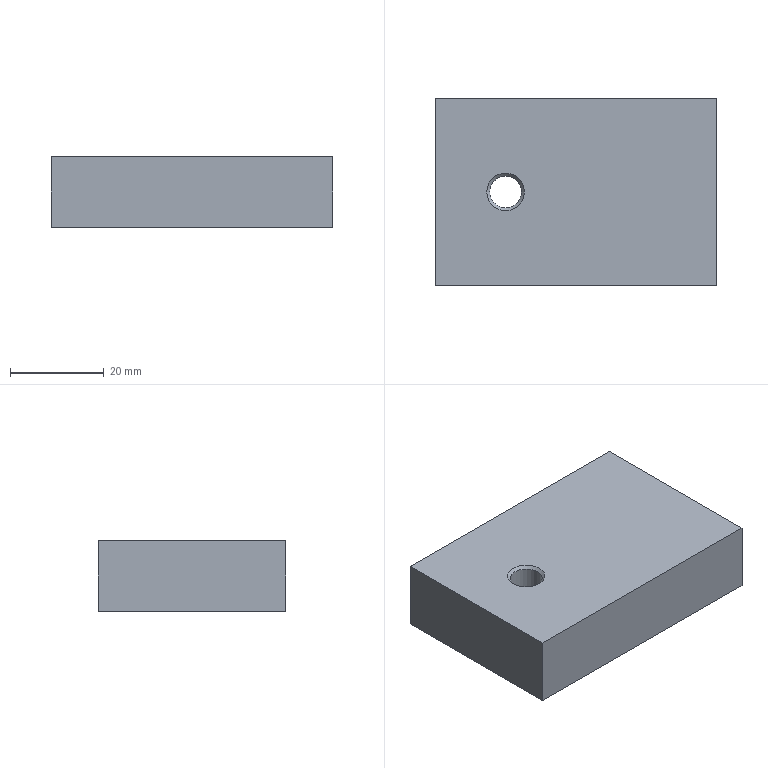Part | NX | features DATUM_CSYS 2, BLOCK 1, HOLE PACKAGE 1, SIMPLE HOLE 1, SKETCH 1, SYMBOLIC_THREAD 1 | 1 solid | 9 faces | box 60 x 40 x 15 mm | volume 35447 mm3 | plane 6 | cone 2 | cylinder 1 | commonest cylinder face diameters 6.8 x1
STEP:
#1=CARTESIAN_POINT('',(19.,20.,15.));
#2=VERTEX_POINT('',#1);
#3=CARTESIAN_POINT('',(15.,20.,15.));
#4=DIRECTION('',(0.,0.,1.));
#5=DIRECTION('',(1.,0.,0.));
#6=AXIS2_PLACEMENT_3D('',#3,#4,#5);
#7=CIRCLE('',#6,4.);
#8=EDGE_CURVE('',#2,#2,#7,.F.);
#9=ORIENTED_EDGE('',*,*,#8,.T.);
#10=EDGE_LOOP('',(#9));
#11=FACE_BOUND('',#10,.T.);
#12=CARTESIAN_POINT('',(60.,0.,15.));
#13=VERTEX_POINT('',#12);
#14=CARTESIAN_POINT('',(0.,0.,15.));
#15=VERTEX_POINT('',#14);
#16=CARTESIAN_POINT('',(30.,0.,15.));
#17=DIRECTION('',(-1.,0.,0.));
#18=VECTOR('',#17,1000.);
#19=LINE('',#16,#18);
#20=EDGE_CURVE('',#13,#15,#19,.T.);
#21=ORIENTED_EDGE('',*,*,#20,.F.);
#22=CARTESIAN_POINT('',(60.,40.,15.));
#23=VERTEX_POINT('',#22);
#24=CARTESIAN_POINT('',(60.,20.,15.));
#25=DIRECTION('',(0.,-1.,0.));
#26=VECTOR('',#25,1000.);
#27=LINE('',#24,#26);
#28=EDGE_CURVE('',#23,#13,#27,.T.);
#29=ORIENTED_EDGE('',*,*,#28,.F.);
#30=CARTESIAN_POINT('',(0.,40.,15.));
#31=VERTEX_POINT('',#30);
#32=CARTESIAN_POINT('',(30.,40.,15.));
#33=DIRECTION('',(1.,0.,0.));
#34=VECTOR('',#33,1000.);
#35=LINE('',#32,#34);
#36=EDGE_CURVE('',#31,#23,#35,.T.);
#37=ORIENTED_EDGE('',*,*,#36,.F.);
#38=CARTESIAN_POINT('',(0.,20.,15.));
#39=DIRECTION('',(0.,1.,0.));
#40=VECTOR('',#39,1000.);
#41=LINE('',#38,#40);
#42=EDGE_CURVE('',#15,#31,#41,.T.);
#43=ORIENTED_EDGE('',*,*,#42,.F.);
#44=EDGE_LOOP('',(#21,#29,#37,#43));
#45=FACE_BOUND('',#44,.T.);
#46=CARTESIAN_POINT('',(30.,20.,15.));
#47=DIRECTION('',(0.,0.,1.));
#48=DIRECTION('',(1.,0.,0.));
#49=AXIS2_PLACEMENT_3D('',#46,#47,#48);
#50=PLANE('',#49);
#51=ADVANCED_FACE('',(#11,#45),#50,.T.);
#52=CARTESIAN_POINT('',(60.,0.,0.));
#53=VERTEX_POINT('',#52);
#54=CARTESIAN_POINT('',(60.,0.,0.));
#55=DIRECTION('',(0.,0.,1.));
#56=VECTOR('',#55,1000.);
#57=LINE('',#54,#56);
#58=EDGE_CURVE('',#53,#13,#57,.T.);
#59=ORIENTED_EDGE('',*,*,#58,.T.);
#60=ORIENTED_EDGE('',*,*,#20,.T.);
#61=CARTESIAN_POINT('',(0.,0.,0.));
#62=VERTEX_POINT('',#61);
#63=CARTESIAN_POINT('',(0.,0.,0.));
#64=DIRECTION('',(0.,0.,1.));
#65=VECTOR('',#64,1000.);
#66=LINE('',#63,#65);
#67=EDGE_CURVE('',#62,#15,#66,.T.);
#68=ORIENTED_EDGE('',*,*,#67,.F.);
#69=CARTESIAN_POINT('',(30.,0.,0.));
#70=DIRECTION('',(1.,0.,0.));
#71=VECTOR('',#70,1000.);
#72=LINE('',#69,#71);
#73=EDGE_CURVE('',#62,#53,#72,.T.);
#74=ORIENTED_EDGE('',*,*,#73,.T.);
#75=EDGE_LOOP('',(#59,#60,#68,#74));
#76=FACE_BOUND('',#75,.T.);
#77=CARTESIAN_POINT('',(30.,0.,0.));
#78=DIRECTION('',(0.,-1.,0.));
#79=DIRECTION('',(0.,0.,-1.));
#80=AXIS2_PLACEMENT_3D('',#77,#78,#79);
#81=PLANE('',#80);
#82=ADVANCED_FACE('',(#76),#81,.T.);
#83=ORIENTED_EDGE('',*,*,#67,.T.);
#84=ORIENTED_EDGE('',*,*,#42,.T.);
#85=CARTESIAN_POINT('',(0.,40.,0.));
#86=VERTEX_POINT('',#85);
#87=CARTESIAN_POINT('',(0.,40.,0.));
#88=DIRECTION('',(0.,0.,1.));
#89=VECTOR('',#88,1000.);
#90=LINE('',#87,#89);
#91=EDGE_CURVE('',#86,#31,#90,.T.);
#92=ORIENTED_EDGE('',*,*,#91,.F.);
#93=CARTESIAN_POINT('',(0.,20.,0.));
#94=DIRECTION('',(0.,-1.,0.));
#95=VECTOR('',#94,1000.);
#96=LINE('',#93,#95);
#97=EDGE_CURVE('',#86,#62,#96,.T.);
#98=ORIENTED_EDGE('',*,*,#97,.T.);
#99=EDGE_LOOP('',(#83,#84,#92,#98));
#100=FACE_BOUND('',#99,.T.);
#101=CARTESIAN_POINT('',(0.,20.,0.));
#102=DIRECTION('',(-1.,0.,0.));
#103=DIRECTION('',(0.,0.,1.));
#104=AXIS2_PLACEMENT_3D('',#101,#102,#103);
#105=PLANE('',#104);
#106=ADVANCED_FACE('',(#100),#105,.T.);
#107=ORIENTED_EDGE('',*,*,#91,.T.);
#108=ORIENTED_EDGE('',*,*,#36,.T.);
#109=CARTESIAN_POINT('',(60.,40.,0.));
#110=VERTEX_POINT('',#109);
#111=CARTESIAN_POINT('',(60.,40.,0.));
#112=DIRECTION('',(0.,0.,1.));
#113=VECTOR('',#112,1000.);
#114=LINE('',#111,#113);
#115=EDGE_CURVE('',#110,#23,#114,.T.);
#116=ORIENTED_EDGE('',*,*,#115,.F.);
#117=CARTESIAN_POINT('',(30.,40.,0.));
#118=DIRECTION('',(-1.,0.,0.));
#119=VECTOR('',#118,1000.);
#120=LINE('',#117,#119);
#121=EDGE_CURVE('',#110,#86,#120,.T.);
#122=ORIENTED_EDGE('',*,*,#121,.T.);
#123=EDGE_LOOP('',(#107,#108,#116,#122));
#124=FACE_BOUND('',#123,.T.);
#125=CARTESIAN_POINT('',(30.,40.,0.));
#126=DIRECTION('',(0.,1.,0.));
#127=DIRECTION('',(0.,0.,1.));
#128=AXIS2_PLACEMENT_3D('',#125,#126,#127);
#129=PLANE('',#128);
#130=ADVANCED_FACE('',(#124),#129,.T.);
#131=CARTESIAN_POINT('',(11.,20.,0.));
#132=VERTEX_POINT('',#131);
#133=CARTESIAN_POINT('',(15.,20.,0.));
#134=DIRECTION('',(0.,0.,-1.));
#135=DIRECTION('',(-1.,0.,0.));
#136=AXIS2_PLACEMENT_3D('',#133,#134,#135);
#137=CIRCLE('',#136,4.);
#138=EDGE_CURVE('',#132,#132,#137,.F.);
#139=ORIENTED_EDGE('',*,*,#138,.T.);
#140=EDGE_LOOP('',(#139));
#141=FACE_BOUND('',#140,.T.);
#142=CARTESIAN_POINT('',(60.,20.,0.));
#143=DIRECTION('',(0.,1.,0.));
#144=VECTOR('',#143,1000.);
#145=LINE('',#142,#144);
#146=EDGE_CURVE('',#53,#110,#145,.T.);
#147=ORIENTED_EDGE('',*,*,#146,.F.);
#148=ORIENTED_EDGE('',*,*,#73,.F.);
#149=ORIENTED_EDGE('',*,*,#97,.F.);
#150=ORIENTED_EDGE('',*,*,#121,.F.);
#151=EDGE_LOOP('',(#147,#148,#149,#150));
#152=FACE_BOUND('',#151,.T.);
#153=CARTESIAN_POINT('',(30.,20.,0.));
#154=DIRECTION('',(0.,0.,-1.));
#155=DIRECTION('',(-1.,0.,0.));
#156=AXIS2_PLACEMENT_3D('',#153,#154,#155);
#157=PLANE('',#156);
#158=ADVANCED_FACE('',(#141,#152),#157,.T.);
#159=ORIENTED_EDGE('',*,*,#146,.T.);
#160=ORIENTED_EDGE('',*,*,#115,.T.);
#161=ORIENTED_EDGE('',*,*,#28,.T.);
#162=ORIENTED_EDGE('',*,*,#58,.F.);
#163=EDGE_LOOP('',(#159,#160,#161,#162));
#164=FACE_BOUND('',#163,.T.);
#165=CARTESIAN_POINT('',(60.,20.,0.));
#166=DIRECTION('',(1.,0.,0.));
#167=DIRECTION('',(0.,0.,-1.));
#168=AXIS2_PLACEMENT_3D('',#165,#166,#167);
#169=PLANE('',#168);
#170=ADVANCED_FACE('',(#164),#169,.T.);
#171=CARTESIAN_POINT('',(11.6,20.,0.6));
#172=VERTEX_POINT('',#171);
#173=CARTESIAN_POINT('',(15.,20.,0.6));
#174=DIRECTION('',(0.,0.,-1.));
#175=DIRECTION('',(-1.,0.,0.));
#176=AXIS2_PLACEMENT_3D('',#173,#174,#175);
#177=CIRCLE('',#176,3.4);
#178=EDGE_CURVE('',#172,#172,#177,.T.);
#179=ORIENTED_EDGE('',*,*,#178,.T.);
#180=EDGE_LOOP('',(#179));
#181=FACE_BOUND('',#180,.T.);
#182=CARTESIAN_POINT('',(18.4,20.,14.4));
#183=VERTEX_POINT('',#182);
#184=CARTESIAN_POINT('',(15.,20.,14.4));
#185=DIRECTION('',(0.,0.,1.));
#186=DIRECTION('',(1.,0.,0.));
#187=AXIS2_PLACEMENT_3D('',#184,#185,#186);
#188=CIRCLE('',#187,3.4);
#189=EDGE_CURVE('',#183,#183,#188,.T.);
#190=ORIENTED_EDGE('',*,*,#189,.T.);
#191=EDGE_LOOP('',(#190));
#192=FACE_BOUND('',#191,.T.);
#193=CARTESIAN_POINT('',(15.,20.,15.));
#194=DIRECTION('',(0.,0.,-1.));
#195=DIRECTION('',(-1.,0.,0.));
#196=AXIS2_PLACEMENT_3D('',#193,#194,#195);
#197=CYLINDRICAL_SURFACE('',#196,3.4);
#198=ADVANCED_FACE('',(#181,#192),#197,.F.);
#199=ORIENTED_EDGE('',*,*,#189,.F.);
#200=EDGE_LOOP('',(#199));
#201=FACE_BOUND('',#200,.T.);
#202=ORIENTED_EDGE('',*,*,#8,.F.);
#203=EDGE_LOOP('',(#202));
#204=FACE_BOUND('',#203,.T.);
#205=CARTESIAN_POINT('',(15.,20.,15.));
#206=DIRECTION('',(0.,0.,1.));
#207=DIRECTION('',(1.,0.,0.));
#208=AXIS2_PLACEMENT_3D('',#205,#206,#207);
#209=CONICAL_SURFACE('',#208,4.,0.7854);
#210=ADVANCED_FACE('',(#201,#204),#209,.F.);
#211=ORIENTED_EDGE('',*,*,#138,.F.);
#212=EDGE_LOOP('',(#211));
#213=FACE_BOUND('',#212,.T.);
#214=ORIENTED_EDGE('',*,*,#178,.F.);
#215=EDGE_LOOP('',(#214));
#216=FACE_BOUND('',#215,.T.);
#217=CARTESIAN_POINT('',(15.,20.,0.6));
#218=DIRECTION('',(0.,0.,-1.));
#219=DIRECTION('',(-1.,0.,0.));
#220=AXIS2_PLACEMENT_3D('',#217,#218,#219);
#221=CONICAL_SURFACE('',#220,3.4,0.7854);
#222=ADVANCED_FACE('',(#213,#216),#221,.F.);
#223=CLOSED_SHELL('',(#51,#82,#106,#130,#158,#170,#198,#210,#222));
#224=MANIFOLD_SOLID_BREP('',#223);
#225=(LENGTH_UNIT()NAMED_UNIT(*)SI_UNIT(.MILLI.,.METRE.));
#226=UNCERTAINTY_MEASURE_WITH_UNIT(LENGTH_MEASURE(0.00001),#225,'','');
#227=(NAMED_UNIT(*)PLANE_ANGLE_UNIT()SI_UNIT($,.RADIAN.));
#228=(NAMED_UNIT(*)SI_UNIT($,.STERADIAN.)SOLID_ANGLE_UNIT());
#229=(GEOMETRIC_REPRESENTATION_CONTEXT(3)GLOBAL_UNCERTAINTY_ASSIGNED_CONTEXT((#226))GLOBAL_UNIT_ASSIGNED_CONTEXT((#225,#227,#228))REPRESENTATION_CONTEXT('',''));
#230=ADVANCED_BREP_SHAPE_REPRESENTATION('',(#224),#229);